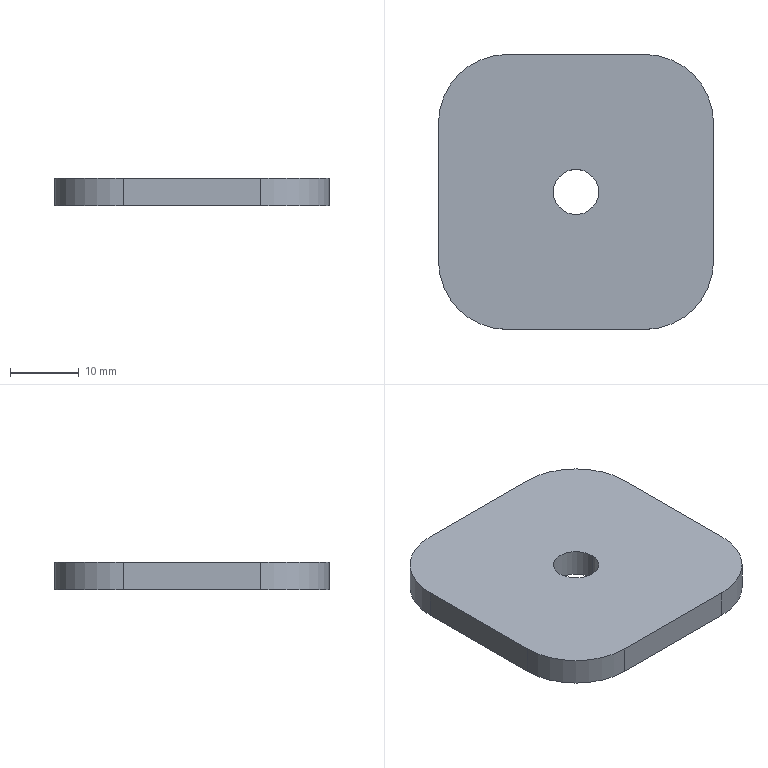Part | SolidWorks | features HoleWzd 3, Extrusion 1, Fillet 1 | 1 solid | 12 faces | box 40 x 40 x 4 mm | volume 5920 mm3 | cylinder 6 | plane 6 | commonest cylinder face diameters 20 x4 6.6 x2
STEP:
#1=CARTESIAN_POINT('',(3.3,0.,4.));
#2=VERTEX_POINT('',#1);
#3=CARTESIAN_POINT('',(-3.3,0.,4.));
#4=VERTEX_POINT('',#3);
#5=CARTESIAN_POINT('',(0.,0.,4.));
#6=DIRECTION('',(0.,0.,-1.));
#7=DIRECTION('',(-1.,0.,0.));
#8=AXIS2_PLACEMENT_3D('',#5,#6,#7);
#9=CIRCLE('',#8,3.3);
#10=EDGE_CURVE('',#2,#4,#9,.T.);
#11=ORIENTED_EDGE('',*,*,#10,.F.);
#12=CARTESIAN_POINT('',(3.3,0.,0.));
#13=VERTEX_POINT('',#12);
#14=CARTESIAN_POINT('',(3.3,0.,0.));
#15=DIRECTION('',(0.,0.,-1.));
#16=VECTOR('',#15,1000.);
#17=LINE('',#14,#16);
#18=EDGE_CURVE('',#2,#13,#17,.T.);
#19=ORIENTED_EDGE('',*,*,#18,.T.);
#20=CARTESIAN_POINT('',(-3.3,0.,0.));
#21=VERTEX_POINT('',#20);
#22=CARTESIAN_POINT('',(0.,0.,0.));
#23=DIRECTION('',(0.,0.,-1.));
#24=DIRECTION('',(-1.,0.,0.));
#25=AXIS2_PLACEMENT_3D('',#22,#23,#24);
#26=CIRCLE('',#25,3.3);
#27=EDGE_CURVE('',#13,#21,#26,.T.);
#28=ORIENTED_EDGE('',*,*,#27,.T.);
#29=CARTESIAN_POINT('',(-3.3,0.,0.));
#30=DIRECTION('',(0.,0.,-1.));
#31=VECTOR('',#30,1000.);
#32=LINE('',#29,#31);
#33=EDGE_CURVE('',#4,#21,#32,.T.);
#34=ORIENTED_EDGE('',*,*,#33,.F.);
#35=EDGE_LOOP('',(#11,#19,#28,#34));
#36=FACE_OUTER_BOUND('',#35,.T.);
#37=CARTESIAN_POINT('',(0.,0.,0.));
#38=DIRECTION('',(0.,0.,-1.));
#39=DIRECTION('',(-1.,0.,0.));
#40=AXIS2_PLACEMENT_3D('',#37,#38,#39);
#41=CYLINDRICAL_SURFACE('',#40,3.3);
#42=ADVANCED_FACE('',(#36),#41,.F.);
#43=CARTESIAN_POINT('',(20.,-10.,0.));
#44=VERTEX_POINT('',#43);
#45=CARTESIAN_POINT('',(20.,10.,0.));
#46=VERTEX_POINT('',#45);
#47=CARTESIAN_POINT('',(20.,20.,0.));
#48=DIRECTION('',(0.,1.,0.));
#49=VECTOR('',#48,1000.);
#50=LINE('',#47,#49);
#51=EDGE_CURVE('',#44,#46,#50,.T.);
#52=ORIENTED_EDGE('',*,*,#51,.T.);
#53=CARTESIAN_POINT('',(20.,10.,4.));
#54=VERTEX_POINT('',#53);
#55=CARTESIAN_POINT('',(20.,10.,4.));
#56=DIRECTION('',(0.,0.,1.));
#57=VECTOR('',#56,1000.);
#58=LINE('',#55,#57);
#59=EDGE_CURVE('',#46,#54,#58,.T.);
#60=ORIENTED_EDGE('',*,*,#59,.T.);
#61=CARTESIAN_POINT('',(20.,-10.,4.));
#62=VERTEX_POINT('',#61);
#63=CARTESIAN_POINT('',(20.,20.,4.));
#64=DIRECTION('',(0.,1.,0.));
#65=VECTOR('',#64,1000.);
#66=LINE('',#63,#65);
#67=EDGE_CURVE('',#62,#54,#66,.T.);
#68=ORIENTED_EDGE('',*,*,#67,.F.);
#69=CARTESIAN_POINT('',(20.,-10.,4.));
#70=DIRECTION('',(0.,0.,-1.));
#71=VECTOR('',#70,1000.);
#72=LINE('',#69,#71);
#73=EDGE_CURVE('',#62,#44,#72,.T.);
#74=ORIENTED_EDGE('',*,*,#73,.T.);
#75=EDGE_LOOP('',(#52,#60,#68,#74));
#76=FACE_OUTER_BOUND('',#75,.T.);
#77=CARTESIAN_POINT('',(20.,20.,4.));
#78=DIRECTION('',(-1.,0.,0.));
#79=DIRECTION('',(0.,-1.,0.));
#80=AXIS2_PLACEMENT_3D('',#77,#78,#79);
#81=PLANE('',#80);
#82=ADVANCED_FACE('',(#76),#81,.F.);
#83=CARTESIAN_POINT('',(10.,20.,4.));
#84=VERTEX_POINT('',#83);
#85=CARTESIAN_POINT('',(-10.,20.,4.));
#86=VERTEX_POINT('',#85);
#87=CARTESIAN_POINT('',(-20.,20.,4.));
#88=DIRECTION('',(-1.,0.,0.));
#89=VECTOR('',#88,1000.);
#90=LINE('',#87,#89);
#91=EDGE_CURVE('',#84,#86,#90,.T.);
#92=ORIENTED_EDGE('',*,*,#91,.F.);
#93=CARTESIAN_POINT('',(10.,20.,0.));
#94=VERTEX_POINT('',#93);
#95=CARTESIAN_POINT('',(10.,20.,4.));
#96=DIRECTION('',(0.,0.,-1.));
#97=VECTOR('',#96,1000.);
#98=LINE('',#95,#97);
#99=EDGE_CURVE('',#84,#94,#98,.T.);
#100=ORIENTED_EDGE('',*,*,#99,.T.);
#101=CARTESIAN_POINT('',(-10.,20.,0.));
#102=VERTEX_POINT('',#101);
#103=CARTESIAN_POINT('',(-20.,20.,0.));
#104=DIRECTION('',(-1.,0.,0.));
#105=VECTOR('',#104,1000.);
#106=LINE('',#103,#105);
#107=EDGE_CURVE('',#94,#102,#106,.T.);
#108=ORIENTED_EDGE('',*,*,#107,.T.);
#109=CARTESIAN_POINT('',(-10.,20.,4.));
#110=DIRECTION('',(0.,0.,1.));
#111=VECTOR('',#110,1000.);
#112=LINE('',#109,#111);
#113=EDGE_CURVE('',#102,#86,#112,.T.);
#114=ORIENTED_EDGE('',*,*,#113,.T.);
#115=EDGE_LOOP('',(#92,#100,#108,#114));
#116=FACE_OUTER_BOUND('',#115,.T.);
#117=CARTESIAN_POINT('',(-20.,20.,4.));
#118=DIRECTION('',(0.,-1.,0.));
#119=DIRECTION('',(0.,0.,-1.));
#120=AXIS2_PLACEMENT_3D('',#117,#118,#119);
#121=PLANE('',#120);
#122=ADVANCED_FACE('',(#116),#121,.F.);
#123=CARTESIAN_POINT('',(-20.,10.,4.));
#124=VERTEX_POINT('',#123);
#125=CARTESIAN_POINT('',(-20.,-10.,4.));
#126=VERTEX_POINT('',#125);
#127=CARTESIAN_POINT('',(-20.,20.,4.));
#128=DIRECTION('',(0.,-1.,0.));
#129=VECTOR('',#128,1000.);
#130=LINE('',#127,#129);
#131=EDGE_CURVE('',#124,#126,#130,.T.);
#132=ORIENTED_EDGE('',*,*,#131,.F.);
#133=CARTESIAN_POINT('',(-20.,10.,0.));
#134=VERTEX_POINT('',#133);
#135=CARTESIAN_POINT('',(-20.,10.,4.));
#136=DIRECTION('',(0.,0.,-1.));
#137=VECTOR('',#136,1000.);
#138=LINE('',#135,#137);
#139=EDGE_CURVE('',#124,#134,#138,.T.);
#140=ORIENTED_EDGE('',*,*,#139,.T.);
#141=CARTESIAN_POINT('',(-20.,-10.,0.));
#142=VERTEX_POINT('',#141);
#143=CARTESIAN_POINT('',(-20.,20.,0.));
#144=DIRECTION('',(0.,-1.,0.));
#145=VECTOR('',#144,1000.);
#146=LINE('',#143,#145);
#147=EDGE_CURVE('',#134,#142,#146,.T.);
#148=ORIENTED_EDGE('',*,*,#147,.T.);
#149=CARTESIAN_POINT('',(-20.,-10.,4.));
#150=DIRECTION('',(0.,0.,1.));
#151=VECTOR('',#150,1000.);
#152=LINE('',#149,#151);
#153=EDGE_CURVE('',#142,#126,#152,.T.);
#154=ORIENTED_EDGE('',*,*,#153,.T.);
#155=EDGE_LOOP('',(#132,#140,#148,#154));
#156=FACE_OUTER_BOUND('',#155,.T.);
#157=CARTESIAN_POINT('',(-20.,20.,4.));
#158=DIRECTION('',(1.,0.,0.));
#159=DIRECTION('',(0.,1.,0.));
#160=AXIS2_PLACEMENT_3D('',#157,#158,#159);
#161=PLANE('',#160);
#162=ADVANCED_FACE('',(#156),#161,.F.);
#163=CARTESIAN_POINT('',(-10.,-20.,0.));
#164=VERTEX_POINT('',#163);
#165=CARTESIAN_POINT('',(10.,-20.,0.));
#166=VERTEX_POINT('',#165);
#167=CARTESIAN_POINT('',(-20.,-20.,0.));
#168=DIRECTION('',(1.,0.,0.));
#169=VECTOR('',#168,1000.);
#170=LINE('',#167,#169);
#171=EDGE_CURVE('',#164,#166,#170,.T.);
#172=ORIENTED_EDGE('',*,*,#171,.T.);
#173=CARTESIAN_POINT('',(10.,-20.,4.));
#174=VERTEX_POINT('',#173);
#175=CARTESIAN_POINT('',(10.,-20.,4.));
#176=DIRECTION('',(0.,0.,1.));
#177=VECTOR('',#176,1000.);
#178=LINE('',#175,#177);
#179=EDGE_CURVE('',#166,#174,#178,.T.);
#180=ORIENTED_EDGE('',*,*,#179,.T.);
#181=CARTESIAN_POINT('',(-10.,-20.,4.));
#182=VERTEX_POINT('',#181);
#183=CARTESIAN_POINT('',(-20.,-20.,4.));
#184=DIRECTION('',(1.,0.,0.));
#185=VECTOR('',#184,1000.);
#186=LINE('',#183,#185);
#187=EDGE_CURVE('',#182,#174,#186,.T.);
#188=ORIENTED_EDGE('',*,*,#187,.F.);
#189=CARTESIAN_POINT('',(-10.,-20.,4.));
#190=DIRECTION('',(0.,0.,-1.));
#191=VECTOR('',#190,1000.);
#192=LINE('',#189,#191);
#193=EDGE_CURVE('',#182,#164,#192,.T.);
#194=ORIENTED_EDGE('',*,*,#193,.T.);
#195=EDGE_LOOP('',(#172,#180,#188,#194));
#196=FACE_OUTER_BOUND('',#195,.T.);
#197=CARTESIAN_POINT('',(-20.,-20.,4.));
#198=DIRECTION('',(0.,1.,0.));
#199=DIRECTION('',(0.,0.,1.));
#200=AXIS2_PLACEMENT_3D('',#197,#198,#199);
#201=PLANE('',#200);
#202=ADVANCED_FACE('',(#196),#201,.F.);
#203=CARTESIAN_POINT('',(0.,0.,4.));
#204=DIRECTION('',(0.,0.,-1.));
#205=DIRECTION('',(-1.,0.,0.));
#206=AXIS2_PLACEMENT_3D('',#203,#204,#205);
#207=CIRCLE('',#206,3.3);
#208=EDGE_CURVE('',#4,#2,#207,.T.);
#209=ORIENTED_EDGE('',*,*,#208,.T.);
#210=ORIENTED_EDGE('',*,*,#10,.T.);
#211=EDGE_LOOP('',(#209,#210));
#212=FACE_BOUND('',#211,.T.);
#213=ORIENTED_EDGE('',*,*,#67,.T.);
#214=CARTESIAN_POINT('',(10.,10.,4.));
#215=DIRECTION('',(0.,0.,1.));
#216=DIRECTION('',(1.,0.,0.));
#217=AXIS2_PLACEMENT_3D('',#214,#215,#216);
#218=CIRCLE('',#217,10.);
#219=EDGE_CURVE('',#54,#84,#218,.T.);
#220=ORIENTED_EDGE('',*,*,#219,.T.);
#221=ORIENTED_EDGE('',*,*,#91,.T.);
#222=CARTESIAN_POINT('',(-10.,10.,4.));
#223=DIRECTION('',(0.,0.,1.));
#224=DIRECTION('',(1.,0.,0.));
#225=AXIS2_PLACEMENT_3D('',#222,#223,#224);
#226=CIRCLE('',#225,10.);
#227=EDGE_CURVE('',#86,#124,#226,.T.);
#228=ORIENTED_EDGE('',*,*,#227,.T.);
#229=ORIENTED_EDGE('',*,*,#131,.T.);
#230=CARTESIAN_POINT('',(-10.,-10.,4.));
#231=DIRECTION('',(0.,0.,1.));
#232=DIRECTION('',(1.,0.,0.));
#233=AXIS2_PLACEMENT_3D('',#230,#231,#232);
#234=CIRCLE('',#233,10.);
#235=EDGE_CURVE('',#126,#182,#234,.T.);
#236=ORIENTED_EDGE('',*,*,#235,.T.);
#237=ORIENTED_EDGE('',*,*,#187,.T.);
#238=CARTESIAN_POINT('',(10.,-10.,4.));
#239=DIRECTION('',(0.,0.,1.));
#240=DIRECTION('',(1.,0.,0.));
#241=AXIS2_PLACEMENT_3D('',#238,#239,#240);
#242=CIRCLE('',#241,10.);
#243=EDGE_CURVE('',#174,#62,#242,.T.);
#244=ORIENTED_EDGE('',*,*,#243,.T.);
#245=EDGE_LOOP('',(#213,#220,#221,#228,#229,#236,#237,#244));
#246=FACE_OUTER_BOUND('',#245,.T.);
#247=CARTESIAN_POINT('',(0.,0.,4.));
#248=DIRECTION('',(0.,0.,1.));
#249=DIRECTION('',(1.,0.,0.));
#250=AXIS2_PLACEMENT_3D('',#247,#248,#249);
#251=PLANE('',#250);
#252=ADVANCED_FACE('',(#212,#246),#251,.T.);
#253=CARTESIAN_POINT('',(0.,0.,0.));
#254=DIRECTION('',(0.,0.,-1.));
#255=DIRECTION('',(-1.,0.,0.));
#256=AXIS2_PLACEMENT_3D('',#253,#254,#255);
#257=CIRCLE('',#256,3.3);
#258=EDGE_CURVE('',#21,#13,#257,.T.);
#259=ORIENTED_EDGE('',*,*,#258,.F.);
#260=ORIENTED_EDGE('',*,*,#27,.F.);
#261=EDGE_LOOP('',(#259,#260));
#262=FACE_BOUND('',#261,.T.);
#263=ORIENTED_EDGE('',*,*,#107,.F.);
#264=CARTESIAN_POINT('',(10.,10.,0.));
#265=DIRECTION('',(0.,0.,-1.));
#266=DIRECTION('',(1.,0.,0.));
#267=AXIS2_PLACEMENT_3D('',#264,#265,#266);
#268=CIRCLE('',#267,10.);
#269=EDGE_CURVE('',#94,#46,#268,.T.);
#270=ORIENTED_EDGE('',*,*,#269,.T.);
#271=ORIENTED_EDGE('',*,*,#51,.F.);
#272=CARTESIAN_POINT('',(10.,-10.,0.));
#273=DIRECTION('',(0.,0.,-1.));
#274=DIRECTION('',(1.,0.,0.));
#275=AXIS2_PLACEMENT_3D('',#272,#273,#274);
#276=CIRCLE('',#275,10.);
#277=EDGE_CURVE('',#44,#166,#276,.T.);
#278=ORIENTED_EDGE('',*,*,#277,.T.);
#279=ORIENTED_EDGE('',*,*,#171,.F.);
#280=CARTESIAN_POINT('',(-10.,-10.,0.));
#281=DIRECTION('',(0.,0.,-1.));
#282=DIRECTION('',(1.,0.,0.));
#283=AXIS2_PLACEMENT_3D('',#280,#281,#282);
#284=CIRCLE('',#283,10.);
#285=EDGE_CURVE('',#164,#142,#284,.T.);
#286=ORIENTED_EDGE('',*,*,#285,.T.);
#287=ORIENTED_EDGE('',*,*,#147,.F.);
#288=CARTESIAN_POINT('',(-10.,10.,0.));
#289=DIRECTION('',(0.,0.,-1.));
#290=DIRECTION('',(1.,0.,0.));
#291=AXIS2_PLACEMENT_3D('',#288,#289,#290);
#292=CIRCLE('',#291,10.);
#293=EDGE_CURVE('',#134,#102,#292,.T.);
#294=ORIENTED_EDGE('',*,*,#293,.T.);
#295=EDGE_LOOP('',(#263,#270,#271,#278,#279,#286,#287,#294));
#296=FACE_OUTER_BOUND('',#295,.T.);
#297=CARTESIAN_POINT('',(0.,0.,0.));
#298=DIRECTION('',(0.,0.,1.));
#299=DIRECTION('',(1.,0.,0.));
#300=AXIS2_PLACEMENT_3D('',#297,#298,#299);
#301=PLANE('',#300);
#302=ADVANCED_FACE('',(#262,#296),#301,.F.);
#303=ORIENTED_EDGE('',*,*,#219,.F.);
#304=ORIENTED_EDGE('',*,*,#59,.F.);
#305=ORIENTED_EDGE('',*,*,#269,.F.);
#306=ORIENTED_EDGE('',*,*,#99,.F.);
#307=EDGE_LOOP('',(#303,#304,#305,#306));
#308=FACE_OUTER_BOUND('',#307,.T.);
#309=CARTESIAN_POINT('',(10.,10.,4.));
#310=DIRECTION('',(0.,0.,-1.));
#311=DIRECTION('',(-1.,0.,0.));
#312=AXIS2_PLACEMENT_3D('',#309,#310,#311);
#313=CYLINDRICAL_SURFACE('',#312,10.);
#314=ADVANCED_FACE('',(#308),#313,.T.);
#315=ORIENTED_EDGE('',*,*,#243,.F.);
#316=ORIENTED_EDGE('',*,*,#179,.F.);
#317=ORIENTED_EDGE('',*,*,#277,.F.);
#318=ORIENTED_EDGE('',*,*,#73,.F.);
#319=EDGE_LOOP('',(#315,#316,#317,#318));
#320=FACE_OUTER_BOUND('',#319,.T.);
#321=CARTESIAN_POINT('',(10.,-10.,4.));
#322=DIRECTION('',(0.,0.,-1.));
#323=DIRECTION('',(-1.,0.,0.));
#324=AXIS2_PLACEMENT_3D('',#321,#322,#323);
#325=CYLINDRICAL_SURFACE('',#324,10.);
#326=ADVANCED_FACE('',(#320),#325,.T.);
#327=ORIENTED_EDGE('',*,*,#227,.F.);
#328=ORIENTED_EDGE('',*,*,#113,.F.);
#329=ORIENTED_EDGE('',*,*,#293,.F.);
#330=ORIENTED_EDGE('',*,*,#139,.F.);
#331=EDGE_LOOP('',(#327,#328,#329,#330));
#332=FACE_OUTER_BOUND('',#331,.T.);
#333=CARTESIAN_POINT('',(-10.,10.,4.));
#334=DIRECTION('',(0.,0.,-1.));
#335=DIRECTION('',(-1.,0.,0.));
#336=AXIS2_PLACEMENT_3D('',#333,#334,#335);
#337=CYLINDRICAL_SURFACE('',#336,10.);
#338=ADVANCED_FACE('',(#332),#337,.T.);
#339=ORIENTED_EDGE('',*,*,#235,.F.);
#340=ORIENTED_EDGE('',*,*,#153,.F.);
#341=ORIENTED_EDGE('',*,*,#285,.F.);
#342=ORIENTED_EDGE('',*,*,#193,.F.);
#343=EDGE_LOOP('',(#339,#340,#341,#342));
#344=FACE_OUTER_BOUND('',#343,.T.);
#345=CARTESIAN_POINT('',(-10.,-10.,4.));
#346=DIRECTION('',(0.,0.,-1.));
#347=DIRECTION('',(-1.,0.,0.));
#348=AXIS2_PLACEMENT_3D('',#345,#346,#347);
#349=CYLINDRICAL_SURFACE('',#348,10.);
#350=ADVANCED_FACE('',(#344),#349,.T.);
#351=ORIENTED_EDGE('',*,*,#18,.F.);
#352=ORIENTED_EDGE('',*,*,#208,.F.);
#353=ORIENTED_EDGE('',*,*,#33,.T.);
#354=ORIENTED_EDGE('',*,*,#258,.T.);
#355=EDGE_LOOP('',(#351,#352,#353,#354));
#356=FACE_OUTER_BOUND('',#355,.T.);
#357=CARTESIAN_POINT('',(0.,0.,0.));
#358=DIRECTION('',(0.,0.,-1.));
#359=DIRECTION('',(-1.,0.,0.));
#360=AXIS2_PLACEMENT_3D('',#357,#358,#359);
#361=CYLINDRICAL_SURFACE('',#360,3.3);
#362=ADVANCED_FACE('',(#356),#361,.F.);
#363=CLOSED_SHELL('',(#42,#82,#122,#162,#202,#252,#302,#314,#326,#338,#350,#362));
#364=MANIFOLD_SOLID_BREP('',#363);
#365=CARTESIAN_POINT('',(0.,0.,0.));
#366=DIRECTION('',(0.,0.,1.));
#367=DIRECTION('',(1.,0.,0.));
#368=AXIS2_PLACEMENT_3D('',#365,#366,#367);
#369=(LENGTH_UNIT()NAMED_UNIT(*)SI_UNIT(.MILLI.,.METRE.));
#370=UNCERTAINTY_MEASURE_WITH_UNIT(LENGTH_MEASURE(0.00001),#369,'','');
#371=(NAMED_UNIT(*)PLANE_ANGLE_UNIT()SI_UNIT($,.RADIAN.));
#372=(NAMED_UNIT(*)SI_UNIT($,.STERADIAN.)SOLID_ANGLE_UNIT());
#373=(GEOMETRIC_REPRESENTATION_CONTEXT(3)GLOBAL_UNCERTAINTY_ASSIGNED_CONTEXT((#370))GLOBAL_UNIT_ASSIGNED_CONTEXT((#369,#371,#372))REPRESENTATION_CONTEXT('',''));
#374=ADVANCED_BREP_SHAPE_REPRESENTATION('',(#364,#368),#373);